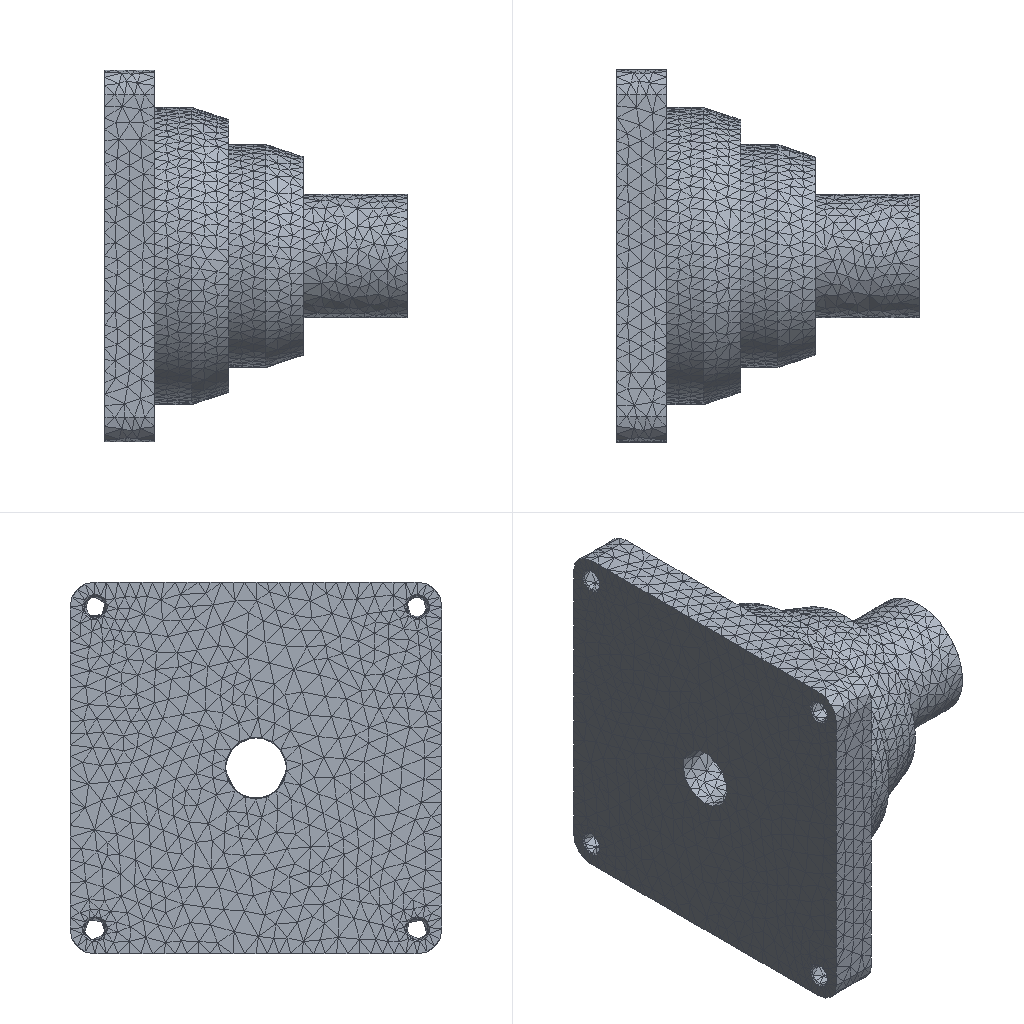Simulation study | ansys workbench
Set-up summary:
category,name,step,type,value,unit,region
solver,ansys_workbench
units,SI m-kg-s (Pa),,stated,"/units,MKS"
analysis,LS1,,static
load_step,LS1,LS1,static,nsubst=1; time=1
mesh,nodes,,,33119
mesh,elements,,,20339
element_type,SOLID187,,,19799
element_type,CONTA174,,,540
material,Structural Steel,,E,2e+11,Pa
material,Structural Steel,,nu,0.3
material,Structural Steel,,density,7850,kg m^-3
material,Structural Steel,,conductivity,60.5,W m^-1 C^-1
material,Structural Steel,,specific_heat,434,J kg^-1 C^-1
material,Structural Steel,,cte,1.2e-05,C^-1
material,Structural Steel,,permeability,10000
material,Structural Steel,,resistivity,1.7e-07,kg m^3 A^-2 s^-3
load,,LS1,moment,"3000 [dir=(0, 1, 0) n=3]",,all
bc,Fixed Supports,model,fixed,[dofs=ALL],,_FIXEDSU
contact,contact 1,,bonded (always),element=CONTA174
named_set,_FIXEDSU,,node,2323
Ansys APDL input file, long lists of numbers shortened:
/batch
/config,noeldb,1     ! force off writing results to database
*get,_wallstrt,active,,time,wall
! ANSYS input file written by Workbench version 2024 R1
! File used for geometry attach:
/title,wbnew--____ (A5)
! ****** Begin Custom Load Command Snippet ******
/COM, ACT Extensions:
/COM,     LSDYNA, 2024.1
/COM,/COM,     ANSYSMotion, 2024.1
/COM,
! ****** End   Custom Load Command Snippet ******
*DIM,_wb_ProjectScratch_dir,string,248
_wb_ProjectScratch_dir(1) = ''
*DIM,_wb_SolverFiles_dir,string,248
_wb_SolverFiles_dir(1) = ''
*DIM,_wb_userfiles_dir,string,248
_wb_userfiles_dir(1) = ''
/com,--- Data in consistent MKS units. See Solving Units in the help system for more information.
/units,MKS
/nopr
/wb,file,start              !  signify a WB generated input file
/prep7
! Turn off shape checking because checks already performed inside WB mesher.
! See help system for more information.
SHPP,OFF,,NOWARN
/nolist
etcon,set             ! allow ANSYS to choose best KEYOP's for 180x elements, resets any applicable keyopt to MAPDL defaults
/com,*********** Nodes for the whole assembly ***********
nblock,3,,36429
(1i9,3e20.9e3)
        1     0.000000000E+00    -7.500000000E-02     6.500000000E-02
! (33117 more lines like these left out)
-1
/com,*********** Nodes for all Remote Points ***********
nblock,3
(1i9,3e20.9e3)
    33119     1.010000000E-01     4.428297363E-06    -1.855682782E-07
-1
/wb,elem,start            !  set before creation of elements
/com,*********** Elements for Body 1 "2012" ***********
et,1,187
eblock,19,solid,,19799
(19i9)
        1        1        1        1        0        0        0        0       10        0        1     3358     5026     4161     4541    25315    30989    25313    25314
! (39597 more lines like these left out)
-1
/wb,elem,end               !  done creating elements
/com,*********** Send User Defined Coordinate System(s) ***********
csys,0
toffst,273.15,  ! Temperature offset from absolute zero
/com,*********** Set Reference Temperature ***********
tref,22.
/wb,mat,start              !  starting to send materials
/com,*********** Send Materials ***********
Temperature = 'TEMP' ! Temperature
MP,DENS,1,7850,	! kg m^-3
MP,ALPX,1,1.2e-05,	! C^-1
MP,C,1,434,	! J kg^-1 C^-1
MP,KXX,1,60.5,	! W m^-1 C^-1
MP,RSVX,1,1.7e-07,	! kg m^3 A^-2 s^-3
MP,EX,1,200000000000,	! Pa
MP,NUXY,1,0.3,
MP,MURX,1,10000,
/wb,mat,end                !  done sending materials
!************************* Model Summary ********************
!2012,	ç»æé¢,	matid,	1
!************************* End Model Summary ********************
! get the diagonal of the bounding box. Needed later for other things
*get,_xmin,node,,mnloc,x
*get,_ymin,node,,mnloc,y
*get,_zmin,node,,mnloc,z
*get,_xmax,node,,mxloc,x
*get,_ymax,node,,mxloc,y
*get,_zmax,node,,mxloc,z
_ASMDIAG=(_xmax-_xmin)*(_xmax-_xmin)+(_ymax-_ymin)*(_ymax-_ymin)+(_zmax-_zmin)*(_zmax-_zmin)
_ASMDIAG=SQRT(_ASMDIAG)
/wb,contact,start          !  starting to send contact
/wb,contact,end            !  done creating contacts
/golist
/wb,load,start             !  starting to send loads
/com,*********** Fixed Supports ***********
CMBLOCK,_FIXEDSU,NODE,     2323
(8i10)
         1         2         3         4         5         6         7         8
! (290 more lines like these left out)
cmsel,s,_FIXEDSU
d,all,all
nsel,all
/com,*********** Create Remote Point "ÄÚ²¿Ô¶³Ìµã" ***********
! -------- Remote Point Used by "Á¦¾Ø" --------
*set,tid,3
*set,cid,2
et,cid,174
et,tid,170
keyo,tid,2,1               ! Don't fix the pilot node
keyo,tid,4,111111
keyo,cid,12,5              ! Bonded Contact
keyo,cid,4,1               ! Deformable RBE3 style load
keyo,cid,2,2               ! MPC style contact
eblock,10,,,540
(15i9)
    26311        2        2        2        0      884      885     2002     2002    11053    11066     2002    11054
! (539 more lines like these left out)
-1
*set,_npilot,33119
_npilot32=_npilot
type,tid
mat ,cid
real,cid
tshape,pilo
en,26851,_npilot
tshape
/com,*********** Construct Moment Using Remote Attachment ***********
/gst,on,on
fini
*get,_numnode,node,0,count
*get,_numelem,elem,0,count
*get, _MAXELEMNUM, elem, 0, NUM, MAX
*get, _MAXNODENUM, node, 0, NUM, MAX
*get, _MAXELEMTYPE, etyp, 0, NUM, MAX
*get, _MAXREALCONST, rcon, 0, NUM, MAX
/go
/wb,load,end               !  done creating loads
/com,--- Number of total nodes = %_numnode%
/com,--- Number of contact elements = 540
/com,--- Number of spring elements = 0
/com,--- Number of bearing elements = 0
/com,--- Number of solid elements = 19799
/com,--- Number of condensed parts = 0
/com,--- Number of total elements = %_numelem%
*get,_wallbsol,active,,time,wall
/com,****************************************************************************
/com,*************************    SOLUTION       ********************************
/com,****************************************************************************
/solu
antype,0                   ! static analysis
_thickRatio=  1     ! Ratio of thick parts in the model
eqsl,pcg,1e-8,,,,,,1
cntr,print,1               ! print out contact info and also make no initial contact an error
cncheck,dmp		!	Enable program controlled contact splitting for distributed memory parallel run
dmpoption,emat,no             ! Don't combine emat file for DANSYS
dmpoption,esav,no             ! Don't combine esav file for DANSYS
nldiag,cont,iter           ! print out contact info each equilibrium iteration
rescontrol,,none                 ! Do not keep any restart files
/com,****************************************************
/com,******************* SOLVE FOR LS 1 OF 1 ****************
nsel,s,node,,33119
f,all,mx,0.
f,all,my,3000.
f,all,mz,0.
nsel,all
/nopr
/gopr
nsub,1,1,1
time,1.
outres,erase
outres,all,none
outres,nsol,all,
outres,rsol,all
outres,eangl,all
outres,etmp,all
outres,veng,all
outres,strs,all,
outres,epel,all,
outres,eppl,all,
outres,cont,all,
! *********** WB SOLVE COMMAND ***********
! check interactive state
*get,ANSINTER_,active,,int
*if,ANSINTER_,ne,0,then
/eof
*endif
solve
/com *************** Write FE CONNECTORS *********
CEWRITE,file,ce,,INTE
/com,****************************************************
/com,*************** FINISHED SOLVE FOR LS 1 *************
*get,_wallasol,active,,time,wall
/nopr
*get,_numnode,node,0,count
*get,_numelem,elem,0,count
*get, _MAXELEMNUM, elem, 0, NUM, MAX
*get, _MAXNODENUM, node, 0, NUM, MAX,,,INTERNAL
*get, _MAXELEMTYPE, etyp, 0, NUM, MAX
*get, _MAXREALCONST, rcon, 0, NUM, MAX
*get,_NSOLTHREADS,active,0,ntfs
*get,_NSOLPROCESSES,active,0,npfs
/gopr
*get,_PCGITER,active,,solu,cgiter
/post1
xmlo,ENCODING,ISO-8859-1
xmlo,parm
/xml,parm,xml
fini
/gopr
*get,_walldone,active,,time,wall
_preptime=(_wallbsol-_wallstrt)*3600
_solvtime=(_wallasol-_wallbsol)*3600
_posttime=(_walldone-_wallasol)*3600
_totaltim=(_walldone-_wallstrt)*3600
*get,_dlbratio,active,0,solu,dlbr
*get,_combtime,active,0,solu,comb
*get,_ssmode,active,0,solu,ssmm
*get,_ndofs,active,0,solu,ndof
*get,_sol_end_time,active,0,set,time
*if,_sol_end_time,eq,1.,then
/fclean				!clean distributed files
*endif
/com,--- Total number of nodes = %_numnode%
/com,--- Total number of elements = %_numelem%
/com,--- Element load balance ratio = %_dlbratio%
/com,--- Time to combine distributed files = %_combtime%
/com,--- Sparse memory mode = %_ssmode%
/com,--- Number of DOF = %_ndofs%
/wb,file,end               ! done with WB generated input
Results summary:
result,analyses[0].index,,,1
result,analyses[0].system,,,SYS
result,analyses[0].deck,,,deck.dat
result,analyses[0].solve_status,,,completed
result,analyses[0].analysis_type,,,static
result,analyses[0].physics,,,mechanical
result,analyses[0].unit_system,,,"MKS: m, kg, N, s, V, A, degC"
result,analyses[0].n_sets,,,1
result,analyses[0].load_steps[0].set,set=1,,1
result,analyses[0].load_steps[0].time_or_freq,set=1,,1
result,analyses[0].load_steps[0].max_displacement_magnitude,set=1,,9.98644e-05
result,analyses[0].load_steps[0].max_von_mises_nodal,set=1,,3.07543e+08
result,analyses[0].load_steps[0].reaction_force_sum_xyz[1],set=1,,8.23466e-05
result,analyses[0].load_steps[0].reaction_force_sum_xyz[2],set=1,,0.0001112
result,analyses[0].load_steps[0].reaction_force_sum_xyz[3],set=1,,6.36696e-06
result,geometry_export[0][0],,,.step
result,geometry_export[0][1],,,ok
result,geometry_export[0][2],,,1